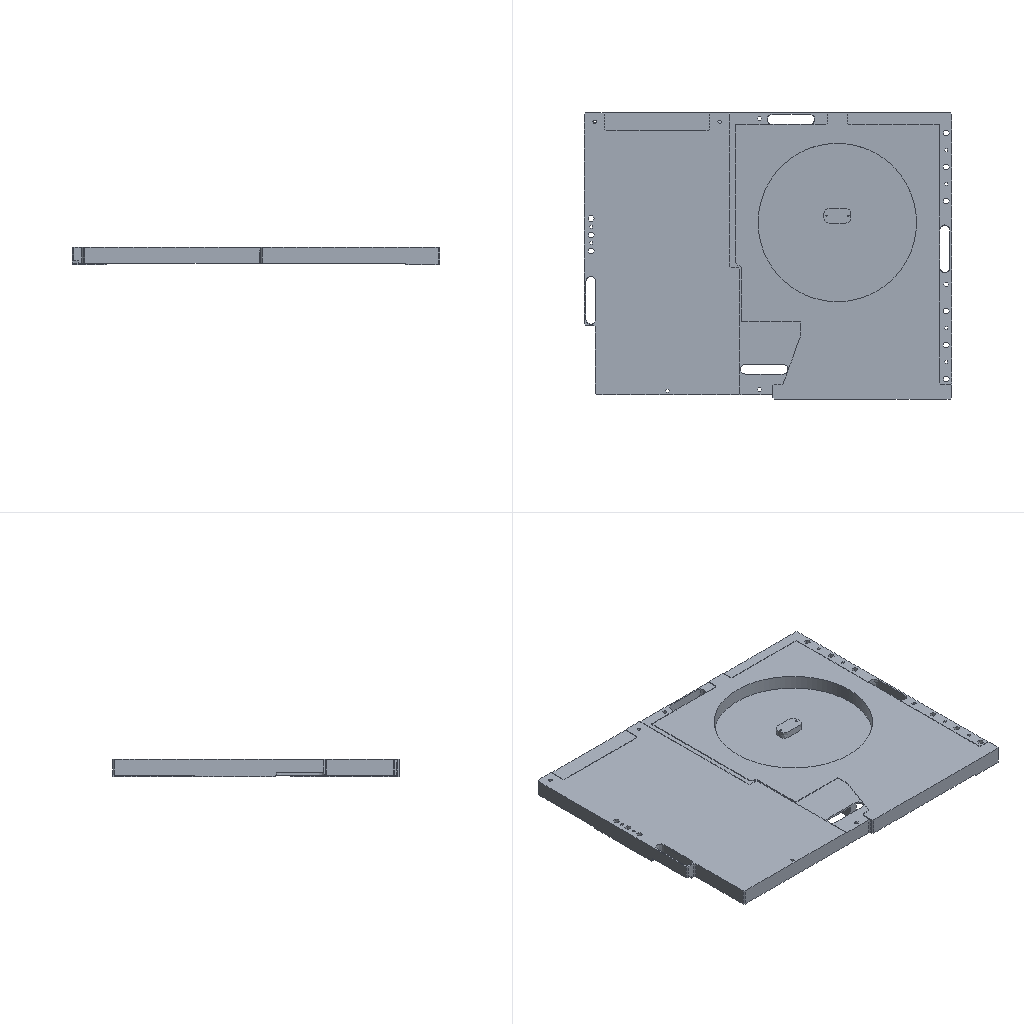Simulation study | nx simcenter
Set-up summary:
category,name,step,type,value,unit,region
solver,nx_nastran (Simcenter)
units,not stated in the deck,,not stated
analysis,deck,,static,static
analysis,solution,,SOL,101
load_step,SUBCASE 1,1,SUBCASE,SPC=1 LOAD=2
load_step,requested,,,1
mesh,nodes,,,127853
mesh,elements,,,68491
element_type,CTETRA,,solid,68491
load,nodal force total,,FX,0.0,model units
load,nodal force total,,FY,0.0,model units
load,nodal force total,,FZ,-2999999.998,model units
load,load commands in deck,,count,10916
bc,support commands in deck,,count,2948
analysis,NX solution 0,,Structural,Linear Statics - Single Constraint
check,setup vs results,,match,every grid point's frame and coordinates and every element id; grid points of CTETRA elements
Nastran input file, long lists of numbers shortened:
$*$$$$$$$$$$$$$$$$$$$$$$$$$$$$$$$$$$$$$$$$$$$$$$$$$$$$$$$$$$$$$$$$$
$*
$*                    NX v10.0.0.24 TRANSLATOR
$*                    FOR NX NASTRAN VERSION 10.0
$ (33 more lines like these left out)
ASSIGN OUTPUT2='130_sim1-solution_1.op2' UNIT=12
$*
$*$$$$$$$$$$$$$$$$$$$$$$$$$$$$$$$$$$$
$*
$* EXECUTIVE CONTROL
$*
$*$$$$$$$$$$$$$$$$$$$$$$$$$$$$$$$$$$$
$*
ID,NASTRAN,130_sim1-solution_1
SOL 101
CEND
$*
$*$$$$$$$$$$$$$$$$$$$$$$$$$$$$$$$$$$$
$*
$* CASE CONTROL
$*
$*$$$$$$$$$$$$$$$$$$$$$$$$$$$$$$$$$$$
$*
TITLE = Solution 1
ECHO = NONE
SPC = 1
OUTPUT
BCRESULTS(TRACTION,FORCE,PLOT) = ALL
DISPLACEMENT(PLOT) = ALL
ESE(PLOT) = ALL
FORCE(PLOT,CORNER) = ALL
OLOAD(PLOT) = ALL
SPCFORCES(PLOT) = ALL
STRAIN(PLOT,FIBER,CORNER) = ALL
STRESS(PLOT,CORNER) = ALL
$*  NX Step: Subcase - Static Loads 1
SUBCASE 1
LABEL = Subcase - Static Loads 1
LOAD = 2
$*
$*$$$$$$$$$$$$$$$$$$$$$$$$$$$$$$$$$$$
$*
$* BULK DATA
$*
$*$$$$$$$$$$$$$$$$$$$$$$$$$$$$$$$$$$$
$*
BEGIN BULK
$*
$* PARAM CARDS
$*
PARAM      K6ROT100.0000
PARAM     OIBULK     YES
PARAM    OMACHPR     YES
PARAM       POST      -2
PARAM    POSTEXT     YES
PARAM    UNITSYS   MN-MM
$*
$* GRID CARDS
$*
GRID*             127324               0-5.140000000E+02-2.900000000E+02+
*       -3.000000000E+00               0
GRID*             127325               0-5.140000000E+02-2.900000000E+02+
*       -2.300000000E+01               0
$ (255702 more lines like these left out)
$*
$* ELEMENT CARDS
$*
$*  NX Mesh Collector: Solid(1)
$*  NX Mesh: 3d_mesh(1)
CTETRA         1       1       1   74899       2       3    2643    2644+
+           2645    2646    2647    2648
CTETRA         2       1       1       4  105826  105825    2649    2650+
+           2651    2652    2653  105997
$ (136978 more lines like these left out)
$*
$* PROPERTY CARDS
$*
$*  NX Property: PSOLID1
PSOLID         1       1       0                           SMECH
$*
$* MATERIAL CARDS
$*
$*  NX Material: Aluminum_2014
MAT1           17.3119+7        0.3300002.7940-62.1355-5
MATT1          1       1               2               3
TABLEM1        1                                                        +
+        20.00007.3119+7 21.11007.3119+7 23.89007.3119+7 37.78007.3119+7+
+        51.67007.3119+7 65.56007.2429+7 79.44007.2429+7 93.33007.1739+7+
+       107.22007.1049+7121.11007.0359+7135.00006.9670+7148.89006.8980+7+
+       162.78006.8290+7176.67006.6910+7190.56006.6221+7204.44006.4841+7+
+       218.33006.3461+7232.22006.1392+7246.11006.0012+7260.00005.8633+7+
+       273.89005.7253+7287.78005.5184+7301.67005.3804+7315.56005.1735+7+
+       329.44004.9665+7343.33004.7596+7357.22004.6216+7371.11004.4147+7+
+           ENDT
TABLEM1        2                                                        +
+        20.00000.330000 21.11000.330000    ENDT
TABLEM1        3                                                        +
+        20.00002.1600-5 93.33002.2500-5107.22002.2662-5121.11002.2824-5+
+       135.00002.2968-5148.89002.3130-5162.78002.3274-5176.67002.3418-5+
+       190.56002.3544-5204.44002.3688-5218.33002.3814-5232.22002.3958-5+
+       246.11002.4066-5260.00002.4192-5273.89002.4300-5287.78002.4408-5+
+       301.67002.4498-5315.56002.4606-5329.44002.4696-5343.33002.4786-5+
+       357.22002.4876-5371.11002.4984-5385.00002.5110-5398.89002.5254-5+
+       412.78002.5398-5426.67002.5560-5    ENDT
$*
$* LOAD AND CONSTRAINT CARDS
$*
$*  NX Load and Constraint: Fixed(1)
SPC            1   57462  123456  0.0000
SPC            1   57463  123456  0.0000
SPC            1   57464  123456  0.0000
SPC            1   57465  123456  0.0000
$ (2944 more lines like these left out)
$*  NX Load and Constraint: Force(1)
FORCE          2   78862       0316.2813  0.0000  0.0000-1.00000
FORCE          2   78863       0319.5445  0.0000  0.0000-1.00000
FORCE          2   78864       0317.4765  0.0000  0.0000-1.00000
FORCE          2   78865       0318.6971  0.0000  0.0000-1.00000
$ (10912 more lines like these left out)
ENDDATA 902465e2
Results summary:
result,analysis,,,static
result,last_loadstep,,,1
result,primary field,,,displacements
result,max displacement,,,0.197,model units
result,reaction total,,FX,-0.4493,model units
result,reaction total,,FY,-0.09947,model units
result,reaction total,,FZ,3000000.5,model units
result,NX solution 0,,loadcases,1,mm